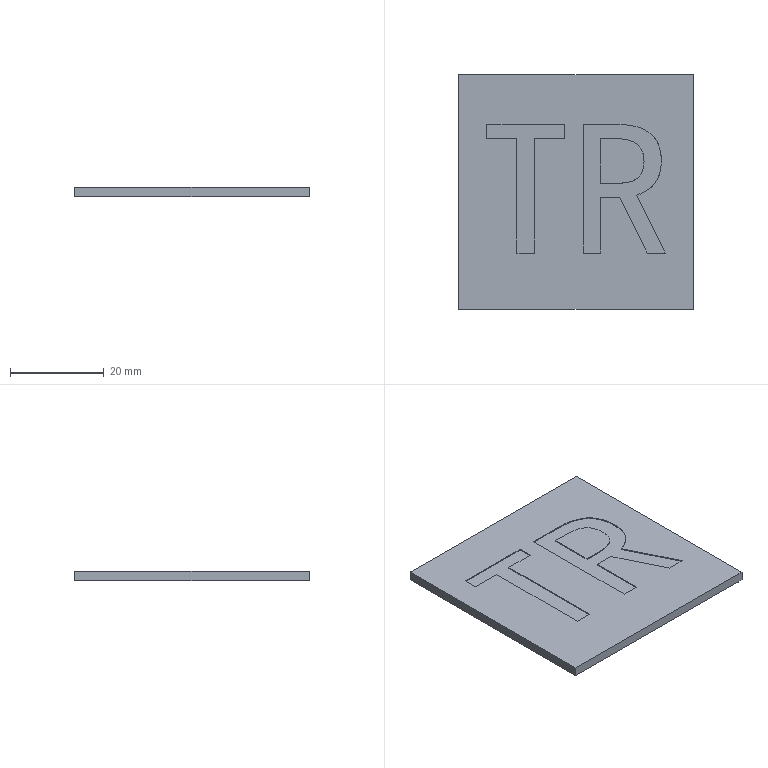Part | STEP file | lll_id986_x_t | 1 solid | 28 faces | box 50 x 50 x 2 mm | volume 4923 mm3 | plane 25 | other 3
STEP:
#1=CARTESIAN_POINT('',(645.037,-531.694,3.259));
#2=VERTEX_POINT('',#1);
#3=CARTESIAN_POINT('',(661.525,-531.694,3.259));
#4=VERTEX_POINT('',#3);
#5=CARTESIAN_POINT('',(653.281,-531.694,3.259));
#6=DIRECTION('',(1.,0.,0.));
#7=VECTOR('',#6,1.);
#8=LINE('',#5,#7);
#9=EDGE_CURVE('',#2,#4,#8,.T.);
#10=ORIENTED_EDGE('',*,*,#9,.T.);
#11=CARTESIAN_POINT('',(661.525,-534.734,3.259));
#12=VERTEX_POINT('',#11);
#13=CARTESIAN_POINT('',(661.525,-533.214,3.259));
#14=DIRECTION('',(0.,-1.,0.));
#15=VECTOR('',#14,1.);
#16=LINE('',#13,#15);
#17=EDGE_CURVE('',#4,#12,#16,.T.);
#18=ORIENTED_EDGE('',*,*,#17,.T.);
#19=CARTESIAN_POINT('',(655.124,-534.734,3.259));
#20=VERTEX_POINT('',#19);
#21=CARTESIAN_POINT('',(658.324,-534.734,3.259));
#22=DIRECTION('',(-1.,0.,0.));
#23=VECTOR('',#22,1.);
#24=LINE('',#21,#23);
#25=EDGE_CURVE('',#12,#20,#24,.T.);
#26=ORIENTED_EDGE('',*,*,#25,.T.);
#27=CARTESIAN_POINT('',(655.124,-559.065,3.259));
#28=VERTEX_POINT('',#27);
#29=CARTESIAN_POINT('',(655.124,-546.899,3.259));
#30=DIRECTION('',(0.,-1.,0.));
#31=VECTOR('',#30,1.);
#32=LINE('',#29,#31);
#33=EDGE_CURVE('',#20,#28,#32,.T.);
#34=ORIENTED_EDGE('',*,*,#33,.T.);
#35=CARTESIAN_POINT('',(651.439,-559.065,3.259));
#36=VERTEX_POINT('',#35);
#37=CARTESIAN_POINT('',(653.281,-559.065,3.259));
#38=DIRECTION('',(-1.,0.,0.));
#39=VECTOR('',#38,1.);
#40=LINE('',#37,#39);
#41=EDGE_CURVE('',#28,#36,#40,.T.);
#42=ORIENTED_EDGE('',*,*,#41,.T.);
#43=CARTESIAN_POINT('',(651.439,-534.734,3.259));
#44=VERTEX_POINT('',#43);
#45=CARTESIAN_POINT('',(651.439,-546.899,3.259));
#46=DIRECTION('',(0.,1.,0.));
#47=VECTOR('',#46,1.);
#48=LINE('',#45,#47);
#49=EDGE_CURVE('',#36,#44,#48,.T.);
#50=ORIENTED_EDGE('',*,*,#49,.T.);
#51=CARTESIAN_POINT('',(645.037,-534.734,3.259));
#52=VERTEX_POINT('',#51);
#53=CARTESIAN_POINT('',(648.238,-534.734,3.259));
#54=DIRECTION('',(-1.,0.,0.));
#55=VECTOR('',#54,1.);
#56=LINE('',#53,#55);
#57=EDGE_CURVE('',#44,#52,#56,.T.);
#58=ORIENTED_EDGE('',*,*,#57,.T.);
#59=CARTESIAN_POINT('',(645.037,-533.214,3.259));
#60=DIRECTION('',(0.,1.,0.));
#61=VECTOR('',#60,1.);
#62=LINE('',#59,#61);
#63=EDGE_CURVE('',#52,#2,#62,.T.);
#64=ORIENTED_EDGE('',*,*,#63,.T.);
#65=EDGE_LOOP('',(#10,#18,#26,#34,#42,#50,#58,#64));
#66=FACE_BOUND('',#65,.T.);
#67=CARTESIAN_POINT('',(689.009,-571.065,3.259));
#68=VERTEX_POINT('',#67);
#69=CARTESIAN_POINT('',(639.009,-571.065,3.259));
#70=VERTEX_POINT('',#69);
#71=CARTESIAN_POINT('',(739.009,-571.065,3.259));
#72=DIRECTION('',(-1.,0.,0.));
#73=VECTOR('',#72,1.);
#74=LINE('',#71,#73);
#75=EDGE_CURVE('',#68,#70,#74,.T.);
#76=ORIENTED_EDGE('',*,*,#75,.F.);
#77=CARTESIAN_POINT('',(689.009,-521.065,3.259));
#78=VERTEX_POINT('',#77);
#79=CARTESIAN_POINT('',(689.009,-471.065,3.259));
#80=DIRECTION('',(0.,-1.,0.));
#81=VECTOR('',#80,1.);
#82=LINE('',#79,#81);
#83=EDGE_CURVE('',#78,#68,#82,.T.);
#84=ORIENTED_EDGE('',*,*,#83,.F.);
#85=CARTESIAN_POINT('',(639.009,-521.065,3.259));
#86=VERTEX_POINT('',#85);
#87=CARTESIAN_POINT('',(739.009,-521.065,3.259));
#88=DIRECTION('',(-1.,0.,0.));
#89=VECTOR('',#88,1.);
#90=LINE('',#87,#89);
#91=EDGE_CURVE('',#78,#86,#90,.T.);
#92=ORIENTED_EDGE('',*,*,#91,.T.);
#93=CARTESIAN_POINT('',(639.009,-471.065,3.259));
#94=DIRECTION('',(0.,1.,0.));
#95=VECTOR('',#94,1.);
#96=LINE('',#93,#95);
#97=EDGE_CURVE('',#70,#86,#96,.T.);
#98=ORIENTED_EDGE('',*,*,#97,.F.);
#99=EDGE_LOOP('',(#76,#84,#92,#98));
#100=FACE_BOUND('',#99,.T.);
#101=CARTESIAN_POINT('',(665.533,-531.694,3.259));
#102=VERTEX_POINT('',#101);
#103=CARTESIAN_POINT('',(676.896,-546.742,3.259));
#104=VERTEX_POINT('',#103);
#105=CARTESIAN_POINT('',(665.533,-531.694,3.259));
#106=CARTESIAN_POINT('',(668.2,-531.694,3.259));
#107=CARTESIAN_POINT('',(670.867,-531.694,3.259));
#108=CARTESIAN_POINT('',(676.1,-531.694,3.259));
#109=CARTESIAN_POINT('',(678.179,-532.302,3.259));
#110=CARTESIAN_POINT('',(681.381,-534.767,3.259));
#111=CARTESIAN_POINT('',(682.179,-536.76,3.259));
#112=CARTESIAN_POINT('',(682.179,-541.668,3.259));
#113=CARTESIAN_POINT('',(681.646,-543.327,3.259));
#114=CARTESIAN_POINT('',(679.511,-545.673,3.259));
#115=CARTESIAN_POINT('',(678.284,-546.419,3.259));
#116=CARTESIAN_POINT('',(676.896,-546.742,3.259));
#117=B_SPLINE_CURVE_WITH_KNOTS('',3,(#105,#106,#107,#108,#109,#110,#111,#112,#113,#114,#115,#116),.UNSPECIFIED.,.F.,.F.,(4,2,2,2,2,4),(0.,0.2266,0.4448,0.6636,0.8315,1.),.UNSPECIFIED.);
#118=EDGE_CURVE('',#102,#104,#117,.T.);
#119=ORIENTED_EDGE('',*,*,#118,.T.);
#120=CARTESIAN_POINT('',(682.982,-559.065,3.259));
#121=VERTEX_POINT('',#120);
#122=CARTESIAN_POINT('',(679.939,-552.903,3.259));
#123=DIRECTION('',(0.4428,-0.8966,0.));
#124=VECTOR('',#123,1.);
#125=LINE('',#122,#124);
#126=EDGE_CURVE('',#104,#121,#125,.T.);
#127=ORIENTED_EDGE('',*,*,#126,.T.);
#128=CARTESIAN_POINT('',(679.14,-559.065,3.259));
#129=VERTEX_POINT('',#128);
#130=CARTESIAN_POINT('',(681.061,-559.065,3.259));
#131=DIRECTION('',(-1.,0.,0.));
#132=VECTOR('',#131,1.);
#133=LINE('',#130,#132);
#134=EDGE_CURVE('',#121,#129,#133,.T.);
#135=ORIENTED_EDGE('',*,*,#134,.T.);
#136=CARTESIAN_POINT('',(673.376,-547.222,3.259));
#137=VERTEX_POINT('',#136);
#138=CARTESIAN_POINT('',(676.258,-553.143,3.259));
#139=DIRECTION('',(-0.4376,0.8992,0.));
#140=VECTOR('',#139,1.);
#141=LINE('',#138,#140);
#142=EDGE_CURVE('',#129,#137,#141,.T.);
#143=ORIENTED_EDGE('',*,*,#142,.T.);
#144=CARTESIAN_POINT('',(669.21,-547.222,3.259));
#145=VERTEX_POINT('',#144);
#146=CARTESIAN_POINT('',(671.293,-547.222,3.259));
#147=DIRECTION('',(-1.,0.,0.));
#148=VECTOR('',#147,1.);
#149=LINE('',#146,#148);
#150=EDGE_CURVE('',#137,#145,#149,.T.);
#151=ORIENTED_EDGE('',*,*,#150,.T.);
#152=CARTESIAN_POINT('',(669.21,-559.065,3.259));
#153=VERTEX_POINT('',#152);
#154=CARTESIAN_POINT('',(669.21,-553.143,3.259));
#155=DIRECTION('',(0.,-1.,0.));
#156=VECTOR('',#155,1.);
#157=LINE('',#154,#156);
#158=EDGE_CURVE('',#145,#153,#157,.T.);
#159=ORIENTED_EDGE('',*,*,#158,.T.);
#160=CARTESIAN_POINT('',(665.533,-559.065,3.259));
#161=VERTEX_POINT('',#160);
#162=CARTESIAN_POINT('',(667.372,-559.065,3.259));
#163=DIRECTION('',(-1.,0.,0.));
#164=VECTOR('',#163,1.);
#165=LINE('',#162,#164);
#166=EDGE_CURVE('',#153,#161,#165,.T.);
#167=ORIENTED_EDGE('',*,*,#166,.T.);
#168=CARTESIAN_POINT('',(665.533,-545.38,3.259));
#169=DIRECTION('',(0.,1.,0.));
#170=VECTOR('',#169,1.);
#171=LINE('',#168,#170);
#172=EDGE_CURVE('',#161,#102,#171,.T.);
#173=ORIENTED_EDGE('',*,*,#172,.T.);
#174=EDGE_LOOP('',(#119,#127,#135,#143,#151,#159,#167,#173));
#175=FACE_BOUND('',#174,.T.);
#176=CARTESIAN_POINT('',(739.009,-471.065,3.259));
#177=DIRECTION('',(0.,0.,1.));
#178=DIRECTION('',(1.,0.,0.));
#179=AXIS2_PLACEMENT_3D('',#176,#177,#178);
#180=PLANE('',#179);
#181=ADVANCED_FACE('',(#66,#100,#175),#180,.T.);
#182=CARTESIAN_POINT('',(689.009,-571.065,1.259));
#183=VERTEX_POINT('',#182);
#184=CARTESIAN_POINT('',(689.009,-571.065,179.534));
#185=DIRECTION('',(0.,0.,1.));
#186=VECTOR('',#185,1.);
#187=LINE('',#184,#186);
#188=EDGE_CURVE('',#183,#68,#187,.T.);
#189=ORIENTED_EDGE('',*,*,#188,.F.);
#190=CARTESIAN_POINT('',(689.009,-521.065,1.259));
#191=VERTEX_POINT('',#190);
#192=CARTESIAN_POINT('',(689.009,-471.065,1.259));
#193=DIRECTION('',(0.,-1.,0.));
#194=VECTOR('',#193,1.);
#195=LINE('',#192,#194);
#196=EDGE_CURVE('',#191,#183,#195,.T.);
#197=ORIENTED_EDGE('',*,*,#196,.F.);
#198=CARTESIAN_POINT('',(689.009,-521.065,2.109));
#199=DIRECTION('',(0.,0.,-1.));
#200=VECTOR('',#199,1.);
#201=LINE('',#198,#200);
#202=EDGE_CURVE('',#78,#191,#201,.T.);
#203=ORIENTED_EDGE('',*,*,#202,.F.);
#204=ORIENTED_EDGE('',*,*,#83,.T.);
#205=EDGE_LOOP('',(#189,#197,#203,#204));
#206=FACE_OUTER_BOUND('',#205,.T.);
#207=CARTESIAN_POINT('',(689.009,-546.065,2.259));
#208=DIRECTION('',(1.,0.,0.));
#209=DIRECTION('',(0.,0.,-1.));
#210=AXIS2_PLACEMENT_3D('',#207,#208,#209);
#211=PLANE('',#210);
#212=ADVANCED_FACE('',(#206),#211,.T.);
#213=CARTESIAN_POINT('',(639.009,-521.065,1.259));
#214=VERTEX_POINT('',#213);
#215=CARTESIAN_POINT('',(639.009,-521.065,2.109));
#216=DIRECTION('',(0.,0.,1.));
#217=VECTOR('',#216,1.);
#218=LINE('',#215,#217);
#219=EDGE_CURVE('',#214,#86,#218,.T.);
#220=ORIENTED_EDGE('',*,*,#219,.F.);
#221=CARTESIAN_POINT('',(639.009,-571.065,1.259));
#222=VERTEX_POINT('',#221);
#223=CARTESIAN_POINT('',(639.009,-471.065,1.259));
#224=DIRECTION('',(0.,-1.,0.));
#225=VECTOR('',#224,1.);
#226=LINE('',#223,#225);
#227=EDGE_CURVE('',#214,#222,#226,.T.);
#228=ORIENTED_EDGE('',*,*,#227,.T.);
#229=CARTESIAN_POINT('',(639.009,-571.065,179.534));
#230=DIRECTION('',(0.,0.,1.));
#231=VECTOR('',#230,1.);
#232=LINE('',#229,#231);
#233=EDGE_CURVE('',#222,#70,#232,.T.);
#234=ORIENTED_EDGE('',*,*,#233,.T.);
#235=ORIENTED_EDGE('',*,*,#97,.T.);
#236=EDGE_LOOP('',(#220,#228,#234,#235));
#237=FACE_OUTER_BOUND('',#236,.T.);
#238=CARTESIAN_POINT('',(639.009,-521.065,2.109));
#239=DIRECTION('',(1.,0.,0.));
#240=DIRECTION('',(0.,0.,-1.));
#241=AXIS2_PLACEMENT_3D('',#238,#239,#240);
#242=PLANE('',#241);
#243=ADVANCED_FACE('',(#237),#242,.F.);
#244=ORIENTED_EDGE('',*,*,#91,.F.);
#245=ORIENTED_EDGE('',*,*,#202,.T.);
#246=CARTESIAN_POINT('',(-820.991,-521.065,1.259));
#247=DIRECTION('',(1.,0.,0.));
#248=VECTOR('',#247,1.);
#249=LINE('',#246,#248);
#250=EDGE_CURVE('',#214,#191,#249,.T.);
#251=ORIENTED_EDGE('',*,*,#250,.F.);
#252=ORIENTED_EDGE('',*,*,#219,.T.);
#253=EDGE_LOOP('',(#244,#245,#251,#252));
#254=FACE_OUTER_BOUND('',#253,.T.);
#255=CARTESIAN_POINT('',(689.009,-521.065,2.109));
#256=DIRECTION('',(0.,1.,0.));
#257=DIRECTION('',(0.,0.,1.));
#258=AXIS2_PLACEMENT_3D('',#255,#256,#257);
#259=PLANE('',#258);
#260=ADVANCED_FACE('',(#254),#259,.T.);
#261=CARTESIAN_POINT('',(-6577.12,-571.065,1.259));
#262=DIRECTION('',(1.,0.,0.));
#263=VECTOR('',#262,1.);
#264=LINE('',#261,#263);
#265=EDGE_CURVE('',#222,#183,#264,.T.);
#266=ORIENTED_EDGE('',*,*,#265,.T.);
#267=ORIENTED_EDGE('',*,*,#188,.T.);
#268=ORIENTED_EDGE('',*,*,#75,.T.);
#269=ORIENTED_EDGE('',*,*,#233,.F.);
#270=EDGE_LOOP('',(#266,#267,#268,#269));
#271=FACE_OUTER_BOUND('',#270,.T.);
#272=CARTESIAN_POINT('',(-6577.12,-571.065,179.534));
#273=DIRECTION('',(0.,-1.,0.));
#274=DIRECTION('',(0.,0.,-1.));
#275=AXIS2_PLACEMENT_3D('',#272,#273,#274);
#276=PLANE('',#275);
#277=ADVANCED_FACE('',(#271),#276,.T.);
#278=ORIENTED_EDGE('',*,*,#250,.T.);
#279=ORIENTED_EDGE('',*,*,#196,.T.);
#280=ORIENTED_EDGE('',*,*,#265,.F.);
#281=ORIENTED_EDGE('',*,*,#227,.F.);
#282=EDGE_LOOP('',(#278,#279,#280,#281));
#283=FACE_OUTER_BOUND('',#282,.T.);
#284=CARTESIAN_POINT('',(-820.991,-471.065,1.259));
#285=DIRECTION('',(0.,0.,-1.));
#286=DIRECTION('',(-1.,0.,0.));
#287=AXIS2_PLACEMENT_3D('',#284,#285,#286);
#288=PLANE('',#287);
#289=ADVANCED_FACE('',(#283),#288,.T.);
#290=ORIENTED_EDGE('',*,*,#17,.F.);
#291=CARTESIAN_POINT('',(661.525,-531.694,3.059));
#292=VERTEX_POINT('',#291);
#293=CARTESIAN_POINT('',(661.525,-531.694,3.059));
#294=DIRECTION('',(0.,0.,-1.));
#295=VECTOR('',#294,1.);
#296=LINE('',#293,#295);
#297=EDGE_CURVE('',#4,#292,#296,.T.);
#298=ORIENTED_EDGE('',*,*,#297,.T.);
#299=CARTESIAN_POINT('',(661.525,-534.734,3.059));
#300=VERTEX_POINT('',#299);
#301=CARTESIAN_POINT('',(661.525,-533.214,3.059));
#302=DIRECTION('',(0.,1.,0.));
#303=VECTOR('',#302,1.);
#304=LINE('',#301,#303);
#305=EDGE_CURVE('',#300,#292,#304,.T.);
#306=ORIENTED_EDGE('',*,*,#305,.F.);
#307=CARTESIAN_POINT('',(661.525,-534.734,3.059));
#308=DIRECTION('',(0.,0.,-1.));
#309=VECTOR('',#308,1.);
#310=LINE('',#307,#309);
#311=EDGE_CURVE('',#12,#300,#310,.T.);
#312=ORIENTED_EDGE('',*,*,#311,.F.);
#313=EDGE_LOOP('',(#290,#298,#306,#312));
#314=FACE_OUTER_BOUND('',#313,.T.);
#315=CARTESIAN_POINT('',(661.525,-531.694,3.059));
#316=DIRECTION('',(-1.,0.,0.));
#317=DIRECTION('',(0.,0.,1.));
#318=AXIS2_PLACEMENT_3D('',#315,#316,#317);
#319=PLANE('',#318);
#320=ADVANCED_FACE('',(#314),#319,.T.);
#321=ORIENTED_EDGE('',*,*,#25,.F.);
#322=ORIENTED_EDGE('',*,*,#311,.T.);
#323=CARTESIAN_POINT('',(655.124,-534.734,3.059));
#324=VERTEX_POINT('',#323);
#325=CARTESIAN_POINT('',(658.324,-534.734,3.059));
#326=DIRECTION('',(1.,0.,0.));
#327=VECTOR('',#326,1.);
#328=LINE('',#325,#327);
#329=EDGE_CURVE('',#324,#300,#328,.T.);
#330=ORIENTED_EDGE('',*,*,#329,.F.);
#331=CARTESIAN_POINT('',(655.124,-534.734,3.059));
#332=DIRECTION('',(0.,0.,-1.));
#333=VECTOR('',#332,1.);
#334=LINE('',#331,#333);
#335=EDGE_CURVE('',#20,#324,#334,.T.);
#336=ORIENTED_EDGE('',*,*,#335,.F.);
#337=EDGE_LOOP('',(#321,#322,#330,#336));
#338=FACE_OUTER_BOUND('',#337,.T.);
#339=CARTESIAN_POINT('',(661.525,-534.734,3.059));
#340=DIRECTION('',(0.,1.,0.));
#341=DIRECTION('',(0.,0.,1.));
#342=AXIS2_PLACEMENT_3D('',#339,#340,#341);
#343=PLANE('',#342);
#344=ADVANCED_FACE('',(#338),#343,.T.);
#345=ORIENTED_EDGE('',*,*,#33,.F.);
#346=ORIENTED_EDGE('',*,*,#335,.T.);
#347=CARTESIAN_POINT('',(655.124,-559.065,3.059));
#348=VERTEX_POINT('',#347);
#349=CARTESIAN_POINT('',(655.124,-546.899,3.059));
#350=DIRECTION('',(0.,1.,0.));
#351=VECTOR('',#350,1.);
#352=LINE('',#349,#351);
#353=EDGE_CURVE('',#348,#324,#352,.T.);
#354=ORIENTED_EDGE('',*,*,#353,.F.);
#355=CARTESIAN_POINT('',(655.124,-559.065,3.059));
#356=DIRECTION('',(0.,0.,-1.));
#357=VECTOR('',#356,1.);
#358=LINE('',#355,#357);
#359=EDGE_CURVE('',#28,#348,#358,.T.);
#360=ORIENTED_EDGE('',*,*,#359,.F.);
#361=EDGE_LOOP('',(#345,#346,#354,#360));
#362=FACE_OUTER_BOUND('',#361,.T.);
#363=CARTESIAN_POINT('',(655.124,-534.734,3.059));
#364=DIRECTION('',(-1.,0.,0.));
#365=DIRECTION('',(0.,0.,1.));
#366=AXIS2_PLACEMENT_3D('',#363,#364,#365);
#367=PLANE('',#366);
#368=ADVANCED_FACE('',(#362),#367,.T.);
#369=ORIENTED_EDGE('',*,*,#41,.F.);
#370=ORIENTED_EDGE('',*,*,#359,.T.);
#371=CARTESIAN_POINT('',(651.439,-559.065,3.059));
#372=VERTEX_POINT('',#371);
#373=CARTESIAN_POINT('',(653.281,-559.065,3.059));
#374=DIRECTION('',(1.,0.,0.));
#375=VECTOR('',#374,1.);
#376=LINE('',#373,#375);
#377=EDGE_CURVE('',#372,#348,#376,.T.);
#378=ORIENTED_EDGE('',*,*,#377,.F.);
#379=CARTESIAN_POINT('',(651.439,-559.065,3.059));
#380=DIRECTION('',(0.,0.,-1.));
#381=VECTOR('',#380,1.);
#382=LINE('',#379,#381);
#383=EDGE_CURVE('',#36,#372,#382,.T.);
#384=ORIENTED_EDGE('',*,*,#383,.F.);
#385=EDGE_LOOP('',(#369,#370,#378,#384));
#386=FACE_OUTER_BOUND('',#385,.T.);
#387=CARTESIAN_POINT('',(655.124,-559.065,3.059));
#388=DIRECTION('',(0.,1.,0.));
#389=DIRECTION('',(0.,0.,1.));
#390=AXIS2_PLACEMENT_3D('',#387,#388,#389);
#391=PLANE('',#390);
#392=ADVANCED_FACE('',(#386),#391,.T.);
#393=ORIENTED_EDGE('',*,*,#49,.F.);
#394=ORIENTED_EDGE('',*,*,#383,.T.);
#395=CARTESIAN_POINT('',(651.439,-534.734,3.059));
#396=VERTEX_POINT('',#395);
#397=CARTESIAN_POINT('',(651.439,-546.899,3.059));
#398=DIRECTION('',(0.,-1.,0.));
#399=VECTOR('',#398,1.);
#400=LINE('',#397,#399);
#401=EDGE_CURVE('',#396,#372,#400,.T.);
#402=ORIENTED_EDGE('',*,*,#401,.F.);
#403=CARTESIAN_POINT('',(651.439,-534.734,3.059));
#404=DIRECTION('',(0.,0.,-1.));
#405=VECTOR('',#404,1.);
#406=LINE('',#403,#405);
#407=EDGE_CURVE('',#44,#396,#406,.T.);
#408=ORIENTED_EDGE('',*,*,#407,.F.);
#409=EDGE_LOOP('',(#393,#394,#402,#408));
#410=FACE_OUTER_BOUND('',#409,.T.);
#411=CARTESIAN_POINT('',(651.439,-559.065,3.059));
#412=DIRECTION('',(1.,0.,0.));
#413=DIRECTION('',(0.,0.,-1.));
#414=AXIS2_PLACEMENT_3D('',#411,#412,#413);
#415=PLANE('',#414);
#416=ADVANCED_FACE('',(#410),#415,.T.);
#417=ORIENTED_EDGE('',*,*,#57,.F.);
#418=ORIENTED_EDGE('',*,*,#407,.T.);
#419=CARTESIAN_POINT('',(645.037,-534.734,3.059));
#420=VERTEX_POINT('',#419);
#421=CARTESIAN_POINT('',(648.238,-534.734,3.059));
#422=DIRECTION('',(1.,0.,0.));
#423=VECTOR('',#422,1.);
#424=LINE('',#421,#423);
#425=EDGE_CURVE('',#420,#396,#424,.T.);
#426=ORIENTED_EDGE('',*,*,#425,.F.);
#427=CARTESIAN_POINT('',(645.037,-534.734,3.059));
#428=DIRECTION('',(0.,0.,-1.));
#429=VECTOR('',#428,1.);
#430=LINE('',#427,#429);
#431=EDGE_CURVE('',#52,#420,#430,.T.);
#432=ORIENTED_EDGE('',*,*,#431,.F.);
#433=EDGE_LOOP('',(#417,#418,#426,#432));
#434=FACE_OUTER_BOUND('',#433,.T.);
#435=CARTESIAN_POINT('',(651.439,-534.734,3.059));
#436=DIRECTION('',(0.,1.,0.));
#437=DIRECTION('',(0.,0.,1.));
#438=AXIS2_PLACEMENT_3D('',#435,#436,#437);
#439=PLANE('',#438);
#440=ADVANCED_FACE('',(#434),#439,.T.);
#441=ORIENTED_EDGE('',*,*,#63,.F.);
#442=ORIENTED_EDGE('',*,*,#431,.T.);
#443=CARTESIAN_POINT('',(645.037,-531.694,3.059));
#444=VERTEX_POINT('',#443);
#445=CARTESIAN_POINT('',(645.037,-533.214,3.059));
#446=DIRECTION('',(0.,-1.,0.));
#447=VECTOR('',#446,1.);
#448=LINE('',#445,#447);
#449=EDGE_CURVE('',#444,#420,#448,.T.);
#450=ORIENTED_EDGE('',*,*,#449,.F.);
#451=CARTESIAN_POINT('',(645.037,-531.694,3.059));
#452=DIRECTION('',(0.,0.,-1.));
#453=VECTOR('',#452,1.);
#454=LINE('',#451,#453);
#455=EDGE_CURVE('',#2,#444,#454,.T.);
#456=ORIENTED_EDGE('',*,*,#455,.F.);
#457=EDGE_LOOP('',(#441,#442,#450,#456));
#458=FACE_OUTER_BOUND('',#457,.T.);
#459=CARTESIAN_POINT('',(645.037,-534.734,3.059));
#460=DIRECTION('',(1.,0.,0.));
#461=DIRECTION('',(0.,0.,-1.));
#462=AXIS2_PLACEMENT_3D('',#459,#460,#461);
#463=PLANE('',#462);
#464=ADVANCED_FACE('',(#458),#463,.T.);
#465=ORIENTED_EDGE('',*,*,#9,.F.);
#466=ORIENTED_EDGE('',*,*,#455,.T.);
#467=CARTESIAN_POINT('',(653.281,-531.694,3.059));
#468=DIRECTION('',(-1.,0.,0.));
#469=VECTOR('',#468,1.);
#470=LINE('',#467,#469);
#471=EDGE_CURVE('',#292,#444,#470,.T.);
#472=ORIENTED_EDGE('',*,*,#471,.F.);
#473=ORIENTED_EDGE('',*,*,#297,.F.);
#474=EDGE_LOOP('',(#465,#466,#472,#473));
#475=FACE_OUTER_BOUND('',#474,.T.);
#476=CARTESIAN_POINT('',(645.037,-531.694,3.059));
#477=DIRECTION('',(0.,-1.,0.));
#478=DIRECTION('',(0.,0.,-1.));
#479=AXIS2_PLACEMENT_3D('',#476,#477,#478);
#480=PLANE('',#479);
#481=ADVANCED_FACE('',(#475),#480,.T.);
#482=ORIENTED_EDGE('',*,*,#305,.T.);
#483=ORIENTED_EDGE('',*,*,#471,.T.);
#484=ORIENTED_EDGE('',*,*,#449,.T.);
#485=ORIENTED_EDGE('',*,*,#425,.T.);
#486=ORIENTED_EDGE('',*,*,#401,.T.);
#487=ORIENTED_EDGE('',*,*,#377,.T.);
#488=ORIENTED_EDGE('',*,*,#353,.T.);
#489=ORIENTED_EDGE('',*,*,#329,.T.);
#490=EDGE_LOOP('',(#482,#483,#484,#485,#486,#487,#488,#489));
#491=FACE_OUTER_BOUND('',#490,.T.);
#492=CARTESIAN_POINT('',(661.525,-533.214,3.059));
#493=DIRECTION('',(0.,0.,1.));
#494=DIRECTION('',(1.,0.,0.));
#495=AXIS2_PLACEMENT_3D('',#492,#493,#494);
#496=PLANE('',#495);
#497=ADVANCED_FACE('',(#491),#496,.T.);
#498=CARTESIAN_POINT('',(677.061,-543.139,3.259));
#499=VERTEX_POINT('',#498);
#500=CARTESIAN_POINT('',(669.21,-534.734,3.259));
#501=VERTEX_POINT('',#500);
#502=CARTESIAN_POINT('',(677.061,-543.139,3.259));
#503=CARTESIAN_POINT('',(678.021,-542.449,3.259));
#504=CARTESIAN_POINT('',(678.502,-541.248,3.259));
#505=CARTESIAN_POINT('',(678.502,-538.043,3.259));
#506=CARTESIAN_POINT('',(678.044,-536.865,3.259));
#507=CARTESIAN_POINT('',(676.224,-535.165,3.259));
#508=CARTESIAN_POINT('',(674.764,-534.734,3.259));
#509=CARTESIAN_POINT('',(671.562,-534.734,3.259));
#510=CARTESIAN_POINT('',(670.386,-534.734,3.259));
#511=CARTESIAN_POINT('',(669.21,-534.734,3.259));
#512=B_SPLINE_CURVE_WITH_KNOTS('',3,(#502,#503,#504,#505,#506,#507,#508,#509,#510,#511),.UNSPECIFIED.,.F.,.F.,(4,2,2,2,4),(0.,0.307,0.5749,0.8439,1.),.UNSPECIFIED.);
#513=EDGE_CURVE('',#499,#501,#512,.T.);
#514=ORIENTED_EDGE('',*,*,#513,.F.);
#515=CARTESIAN_POINT('',(677.061,-543.139,3.059));
#516=VERTEX_POINT('',#515);
#517=CARTESIAN_POINT('',(677.061,-543.139,3.059));
#518=DIRECTION('',(0.,0.,-1.));
#519=VECTOR('',#518,1.);
#520=LINE('',#517,#519);
#521=EDGE_CURVE('',#499,#516,#520,.T.);
#522=ORIENTED_EDGE('',*,*,#521,.T.);
#523=CARTESIAN_POINT('',(669.21,-534.734,3.059));
#524=VERTEX_POINT('',#523);
#525=CARTESIAN_POINT('',(669.21,-534.734,3.059));
#526=CARTESIAN_POINT('',(670.386,-534.734,3.059));
#527=CARTESIAN_POINT('',(671.562,-534.734,3.059));
#528=CARTESIAN_POINT('',(674.764,-534.734,3.059));
#529=CARTESIAN_POINT('',(676.224,-535.165,3.059));
#530=CARTESIAN_POINT('',(678.044,-536.865,3.059));
#531=CARTESIAN_POINT('',(678.502,-538.043,3.059));
#532=CARTESIAN_POINT('',(678.502,-541.248,3.059));
#533=CARTESIAN_POINT('',(678.021,-542.449,3.059));
#534=CARTESIAN_POINT('',(677.061,-543.139,3.059));
#535=B_SPLINE_CURVE_WITH_KNOTS('',3,(#525,#526,#527,#528,#529,#530,#531,#532,#533,#534),.UNSPECIFIED.,.F.,.F.,(4,2,2,2,4),(0.,0.1561,0.4251,0.693,1.),.UNSPECIFIED.);
#536=EDGE_CURVE('',#524,#516,#535,.T.);
#537=ORIENTED_EDGE('',*,*,#536,.F.);
#538=CARTESIAN_POINT('',(669.21,-534.734,3.059));
#539=DIRECTION('',(0.,0.,-1.));
#540=VECTOR('',#539,1.);
#541=LINE('',#538,#540);
#542=EDGE_CURVE('',#501,#524,#541,.T.);
#543=ORIENTED_EDGE('',*,*,#542,.F.);
#544=EDGE_LOOP('',(#514,#522,#537,#543));
#545=FACE_OUTER_BOUND('',#544,.T.);
#546=CARTESIAN_POINT('',(677.061,-543.139,3.059));
#547=CARTESIAN_POINT('',(678.021,-542.449,3.059));
#548=CARTESIAN_POINT('',(678.502,-541.248,3.059));
#549=CARTESIAN_POINT('',(678.502,-538.043,3.059));
#550=CARTESIAN_POINT('',(678.044,-536.865,3.059));
#551=CARTESIAN_POINT('',(676.224,-535.165,3.059));
#552=CARTESIAN_POINT('',(674.764,-534.734,3.059));
#553=CARTESIAN_POINT('',(671.562,-534.734,3.059));
#554=CARTESIAN_POINT('',(670.386,-534.734,3.059));
#555=CARTESIAN_POINT('',(669.21,-534.734,3.059));
#556=B_SPLINE_CURVE_WITH_KNOTS('',3,(#546,#547,#548,#549,#550,#551,#552,#553,#554,#555),.UNSPECIFIED.,.F.,.F.,(4,2,2,2,4),(0.,0.307,0.5749,0.8439,1.),.UNSPECIFIED.);
#557=DIRECTION('',(0.,0.,1.));
#558=VECTOR('',#557,1.);
#559=SURFACE_OF_LINEAR_EXTRUSION('',#556,#558);
#560=ADVANCED_FACE('',(#545),#559,.T.);
#561=CARTESIAN_POINT('',(669.21,-544.182,3.259));
#562=VERTEX_POINT('',#561);
#563=CARTESIAN_POINT('',(669.21,-539.458,3.259));
#564=DIRECTION('',(0.,-1.,0.));
#565=VECTOR('',#564,1.);
#566=LINE('',#563,#565);
#567=EDGE_CURVE('',#501,#562,#566,.T.);
#568=ORIENTED_EDGE('',*,*,#567,.F.);
#569=ORIENTED_EDGE('',*,*,#542,.T.);
#570=CARTESIAN_POINT('',(669.21,-544.182,3.059));
#571=VERTEX_POINT('',#570);
#572=CARTESIAN_POINT('',(669.21,-539.458,3.059));
#573=DIRECTION('',(0.,1.,0.));
#574=VECTOR('',#573,1.);
#575=LINE('',#572,#574);
#576=EDGE_CURVE('',#571,#524,#575,.T.);
#577=ORIENTED_EDGE('',*,*,#576,.F.);
#578=CARTESIAN_POINT('',(669.21,-544.182,3.059));
#579=DIRECTION('',(0.,0.,-1.));
#580=VECTOR('',#579,1.);
#581=LINE('',#578,#580);
#582=EDGE_CURVE('',#562,#571,#581,.T.);
#583=ORIENTED_EDGE('',*,*,#582,.F.);
#584=EDGE_LOOP('',(#568,#569,#577,#583));
#585=FACE_OUTER_BOUND('',#584,.T.);
#586=CARTESIAN_POINT('',(669.21,-534.734,3.059));
#587=DIRECTION('',(-1.,0.,0.));
#588=DIRECTION('',(0.,0.,1.));
#589=AXIS2_PLACEMENT_3D('',#586,#587,#588);
#590=PLANE('',#589);
#591=ADVANCED_FACE('',(#585),#590,.T.);
#592=ORIENTED_EDGE('',*,*,#126,.F.);
#593=CARTESIAN_POINT('',(676.896,-546.742,3.059));
#594=VERTEX_POINT('',#593);
#595=CARTESIAN_POINT('',(676.896,-546.742,3.059));
#596=DIRECTION('',(0.,0.,-1.));
#597=VECTOR('',#596,1.);
#598=LINE('',#595,#597);
#599=EDGE_CURVE('',#104,#594,#598,.T.);
#600=ORIENTED_EDGE('',*,*,#599,.T.);
#601=CARTESIAN_POINT('',(682.982,-559.065,3.059));
#602=VERTEX_POINT('',#601);
#603=CARTESIAN_POINT('',(679.939,-552.903,3.059));
#604=DIRECTION('',(-0.4428,0.8966,0.));
#605=VECTOR('',#604,1.);
#606=LINE('',#603,#605);
#607=EDGE_CURVE('',#602,#594,#606,.T.);
#608=ORIENTED_EDGE('',*,*,#607,.F.);
#609=CARTESIAN_POINT('',(682.982,-559.065,3.059));
#610=DIRECTION('',(0.,0.,-1.));
#611=VECTOR('',#610,1.);
#612=LINE('',#609,#611);
#613=EDGE_CURVE('',#121,#602,#612,.T.);
#614=ORIENTED_EDGE('',*,*,#613,.F.);
#615=EDGE_LOOP('',(#592,#600,#608,#614));
#616=FACE_OUTER_BOUND('',#615,.T.);
#617=CARTESIAN_POINT('',(676.896,-546.742,3.059));
#618=DIRECTION('',(-0.8966,-0.4428,0.));
#619=DIRECTION('',(0.4428,-0.8966,0.));
#620=AXIS2_PLACEMENT_3D('',#617,#618,#619);
#621=PLANE('',#620);
#622=ADVANCED_FACE('',(#616),#621,.T.);
#623=ORIENTED_EDGE('',*,*,#134,.F.);
#624=ORIENTED_EDGE('',*,*,#613,.T.);
#625=CARTESIAN_POINT('',(679.14,-559.065,3.059));
#626=VERTEX_POINT('',#625);
#627=CARTESIAN_POINT('',(681.061,-559.065,3.059));
#628=DIRECTION('',(1.,0.,0.));
#629=VECTOR('',#628,1.);
#630=LINE('',#627,#629);
#631=EDGE_CURVE('',#626,#602,#630,.T.);
#632=ORIENTED_EDGE('',*,*,#631,.F.);
#633=CARTESIAN_POINT('',(679.14,-559.065,3.059));
#634=DIRECTION('',(0.,0.,-1.));
#635=VECTOR('',#634,1.);
#636=LINE('',#633,#635);
#637=EDGE_CURVE('',#129,#626,#636,.T.);
#638=ORIENTED_EDGE('',*,*,#637,.F.);
#639=EDGE_LOOP('',(#623,#624,#632,#638));
#640=FACE_OUTER_BOUND('',#639,.T.);
#641=CARTESIAN_POINT('',(682.982,-559.065,3.059));
#642=DIRECTION('',(0.,1.,0.));
#643=DIRECTION('',(0.,0.,1.));
#644=AXIS2_PLACEMENT_3D('',#641,#642,#643);
#645=PLANE('',#644);
#646=ADVANCED_FACE('',(#640),#645,.T.);
#647=ORIENTED_EDGE('',*,*,#142,.F.);
#648=ORIENTED_EDGE('',*,*,#637,.T.);
#649=CARTESIAN_POINT('',(673.376,-547.222,3.059));
#650=VERTEX_POINT('',#649);
#651=CARTESIAN_POINT('',(676.258,-553.143,3.059));
#652=DIRECTION('',(0.4376,-0.8992,0.));
#653=VECTOR('',#652,1.);
#654=LINE('',#651,#653);
#655=EDGE_CURVE('',#650,#626,#654,.T.);
#656=ORIENTED_EDGE('',*,*,#655,.F.);
#657=CARTESIAN_POINT('',(673.376,-547.222,3.059));
#658=DIRECTION('',(0.,0.,-1.));
#659=VECTOR('',#658,1.);
#660=LINE('',#657,#659);
#661=EDGE_CURVE('',#137,#650,#660,.T.);
#662=ORIENTED_EDGE('',*,*,#661,.F.);
#663=EDGE_LOOP('',(#647,#648,#656,#662));
#664=FACE_OUTER_BOUND('',#663,.T.);
#665=CARTESIAN_POINT('',(679.14,-559.065,3.059));
#666=DIRECTION('',(0.8992,0.4376,0.));
#667=DIRECTION('',(-0.4376,0.8992,0.));
#668=AXIS2_PLACEMENT_3D('',#665,#666,#667);
#669=PLANE('',#668);
#670=ADVANCED_FACE('',(#664),#669,.T.);
#671=ORIENTED_EDGE('',*,*,#150,.F.);
#672=ORIENTED_EDGE('',*,*,#661,.T.);
#673=CARTESIAN_POINT('',(669.21,-547.222,3.059));
#674=VERTEX_POINT('',#673);
#675=CARTESIAN_POINT('',(671.293,-547.222,3.059));
#676=DIRECTION('',(1.,0.,0.));
#677=VECTOR('',#676,1.);
#678=LINE('',#675,#677);
#679=EDGE_CURVE('',#674,#650,#678,.T.);
#680=ORIENTED_EDGE('',*,*,#679,.F.);
#681=CARTESIAN_POINT('',(669.21,-547.222,3.059));
#682=DIRECTION('',(0.,0.,-1.));
#683=VECTOR('',#682,1.);
#684=LINE('',#681,#683);
#685=EDGE_CURVE('',#145,#674,#684,.T.);
#686=ORIENTED_EDGE('',*,*,#685,.F.);
#687=EDGE_LOOP('',(#671,#672,#680,#686));
#688=FACE_OUTER_BOUND('',#687,.T.);
#689=CARTESIAN_POINT('',(673.376,-547.222,3.059));
#690=DIRECTION('',(0.,1.,0.));
#691=DIRECTION('',(0.,0.,1.));
#692=AXIS2_PLACEMENT_3D('',#689,#690,#691);
#693=PLANE('',#692);
#694=ADVANCED_FACE('',(#688),#693,.T.);
#695=ORIENTED_EDGE('',*,*,#158,.F.);
#696=ORIENTED_EDGE('',*,*,#685,.T.);
#697=CARTESIAN_POINT('',(669.21,-559.065,3.059));
#698=VERTEX_POINT('',#697);
#699=CARTESIAN_POINT('',(669.21,-553.143,3.059));
#700=DIRECTION('',(0.,1.,0.));
#701=VECTOR('',#700,1.);
#702=LINE('',#699,#701);
#703=EDGE_CURVE('',#698,#674,#702,.T.);
#704=ORIENTED_EDGE('',*,*,#703,.F.);
#705=CARTESIAN_POINT('',(669.21,-559.065,3.059));
#706=DIRECTION('',(0.,0.,-1.));
#707=VECTOR('',#706,1.);
#708=LINE('',#705,#707);
#709=EDGE_CURVE('',#153,#698,#708,.T.);
#710=ORIENTED_EDGE('',*,*,#709,.F.);
#711=EDGE_LOOP('',(#695,#696,#704,#710));
#712=FACE_OUTER_BOUND('',#711,.T.);
#713=CARTESIAN_POINT('',(669.21,-547.222,3.059));
#714=DIRECTION('',(-1.,0.,0.));
#715=DIRECTION('',(0.,0.,1.));
#716=AXIS2_PLACEMENT_3D('',#713,#714,#715);
#717=PLANE('',#716);
#718=ADVANCED_FACE('',(#712),#717,.T.);
#719=ORIENTED_EDGE('',*,*,#166,.F.);
#720=ORIENTED_EDGE('',*,*,#709,.T.);
#721=CARTESIAN_POINT('',(665.533,-559.065,3.059));
#722=VERTEX_POINT('',#721);
#723=CARTESIAN_POINT('',(667.372,-559.065,3.059));
#724=DIRECTION('',(1.,0.,0.));
#725=VECTOR('',#724,1.);
#726=LINE('',#723,#725);
#727=EDGE_CURVE('',#722,#698,#726,.T.);
#728=ORIENTED_EDGE('',*,*,#727,.F.);
#729=CARTESIAN_POINT('',(665.533,-559.065,3.059));
#730=DIRECTION('',(0.,0.,-1.));
#731=VECTOR('',#730,1.);
#732=LINE('',#729,#731);
#733=EDGE_CURVE('',#161,#722,#732,.T.);
#734=ORIENTED_EDGE('',*,*,#733,.F.);
#735=EDGE_LOOP('',(#719,#720,#728,#734));
#736=FACE_OUTER_BOUND('',#735,.T.);
#737=CARTESIAN_POINT('',(669.21,-559.065,3.059));
#738=DIRECTION('',(0.,1.,0.));
#739=DIRECTION('',(0.,0.,1.));
#740=AXIS2_PLACEMENT_3D('',#737,#738,#739);
#741=PLANE('',#740);
#742=ADVANCED_FACE('',(#736),#741,.T.);
#743=ORIENTED_EDGE('',*,*,#172,.F.);
#744=ORIENTED_EDGE('',*,*,#733,.T.);
#745=CARTESIAN_POINT('',(665.533,-531.694,3.059));
#746=VERTEX_POINT('',#745);
#747=CARTESIAN_POINT('',(665.533,-545.38,3.059));
#748=DIRECTION('',(0.,-1.,0.));
#749=VECTOR('',#748,1.);
#750=LINE('',#747,#749);
#751=EDGE_CURVE('',#746,#722,#750,.T.);
#752=ORIENTED_EDGE('',*,*,#751,.F.);
#753=CARTESIAN_POINT('',(665.533,-531.694,3.059));
#754=DIRECTION('',(0.,0.,-1.));
#755=VECTOR('',#754,1.);
#756=LINE('',#753,#755);
#757=EDGE_CURVE('',#102,#746,#756,.T.);
#758=ORIENTED_EDGE('',*,*,#757,.F.);
#759=EDGE_LOOP('',(#743,#744,#752,#758));
#760=FACE_OUTER_BOUND('',#759,.T.);
#761=CARTESIAN_POINT('',(665.533,-559.065,3.059));
#762=DIRECTION('',(1.,0.,0.));
#763=DIRECTION('',(0.,0.,-1.));
#764=AXIS2_PLACEMENT_3D('',#761,#762,#763);
#765=PLANE('',#764);
#766=ADVANCED_FACE('',(#760),#765,.T.);
#767=ORIENTED_EDGE('',*,*,#118,.F.);
#768=ORIENTED_EDGE('',*,*,#757,.T.);
#769=CARTESIAN_POINT('',(676.896,-546.742,3.059));
#770=CARTESIAN_POINT('',(678.284,-546.419,3.059));
#771=CARTESIAN_POINT('',(679.511,-545.673,3.059));
#772=CARTESIAN_POINT('',(681.646,-543.327,3.059));
#773=CARTESIAN_POINT('',(682.179,-541.668,3.059));
#774=CARTESIAN_POINT('',(682.179,-536.76,3.059));
#775=CARTESIAN_POINT('',(681.381,-534.767,3.059));
#776=CARTESIAN_POINT('',(678.179,-532.302,3.059));
#777=CARTESIAN_POINT('',(676.1,-531.694,3.059));
#778=CARTESIAN_POINT('',(670.867,-531.694,3.059));
#779=CARTESIAN_POINT('',(668.2,-531.694,3.059));
#780=CARTESIAN_POINT('',(665.533,-531.694,3.059));
#781=B_SPLINE_CURVE_WITH_KNOTS('',3,(#769,#770,#771,#772,#773,#774,#775,#776,#777,#778,#779,#780),.UNSPECIFIED.,.F.,.F.,(4,2,2,2,2,4),(0.,0.1685,0.3364,0.5552,0.7734,1.),.UNSPECIFIED.);
#782=EDGE_CURVE('',#594,#746,#781,.T.);
#783=ORIENTED_EDGE('',*,*,#782,.F.);
#784=ORIENTED_EDGE('',*,*,#599,.F.);
#785=EDGE_LOOP('',(#767,#768,#783,#784));
#786=FACE_OUTER_BOUND('',#785,.T.);
#787=CARTESIAN_POINT('',(665.533,-531.694,3.059));
#788=CARTESIAN_POINT('',(668.2,-531.694,3.059));
#789=CARTESIAN_POINT('',(670.867,-531.694,3.059));
#790=CARTESIAN_POINT('',(676.1,-531.694,3.059));
#791=CARTESIAN_POINT('',(678.179,-532.302,3.059));
#792=CARTESIAN_POINT('',(681.381,-534.767,3.059));
#793=CARTESIAN_POINT('',(682.179,-536.76,3.059));
#794=CARTESIAN_POINT('',(682.179,-541.668,3.059));
#795=CARTESIAN_POINT('',(681.646,-543.327,3.059));
#796=CARTESIAN_POINT('',(679.511,-545.673,3.059));
#797=CARTESIAN_POINT('',(678.284,-546.419,3.059));
#798=CARTESIAN_POINT('',(676.896,-546.742,3.059));
#799=B_SPLINE_CURVE_WITH_KNOTS('',3,(#787,#788,#789,#790,#791,#792,#793,#794,#795,#796,#797,#798),.UNSPECIFIED.,.F.,.F.,(4,2,2,2,2,4),(0.,0.2266,0.4448,0.6636,0.8315,1.),.UNSPECIFIED.);
#800=DIRECTION('',(0.,0.,1.));
#801=VECTOR('',#800,1.);
#802=SURFACE_OF_LINEAR_EXTRUSION('',#799,#801);
#803=ADVANCED_FACE('',(#786),#802,.T.);
#804=CARTESIAN_POINT('',(669.21,-544.182,3.259));
#805=CARTESIAN_POINT('',(670.706,-544.182,3.259));
#806=CARTESIAN_POINT('',(672.202,-544.182,3.259));
#807=CARTESIAN_POINT('',(674.974,-544.182,3.259));
#808=CARTESIAN_POINT('',(676.1,-543.83,3.259));
#809=CARTESIAN_POINT('',(677.061,-543.139,3.259));
#810=B_SPLINE_CURVE_WITH_KNOTS('',3,(#804,#805,#806,#807,#808,#809),.UNSPECIFIED.,.F.,.F.,(4,2,4),(0.,0.5397,1.),.UNSPECIFIED.);
#811=EDGE_CURVE('',#562,#499,#810,.T.);
#812=ORIENTED_EDGE('',*,*,#811,.F.);
#813=ORIENTED_EDGE('',*,*,#582,.T.);
#814=CARTESIAN_POINT('',(677.061,-543.139,3.059));
#815=CARTESIAN_POINT('',(676.1,-543.83,3.059));
#816=CARTESIAN_POINT('',(674.974,-544.182,3.059));
#817=CARTESIAN_POINT('',(672.202,-544.182,3.059));
#818=CARTESIAN_POINT('',(670.706,-544.182,3.059));
#819=CARTESIAN_POINT('',(669.21,-544.182,3.059));
#820=B_SPLINE_CURVE_WITH_KNOTS('',3,(#814,#815,#816,#817,#818,#819),.UNSPECIFIED.,.F.,.F.,(4,2,4),(0.,0.4603,1.),.UNSPECIFIED.);
#821=EDGE_CURVE('',#516,#571,#820,.T.);
#822=ORIENTED_EDGE('',*,*,#821,.F.);
#823=ORIENTED_EDGE('',*,*,#521,.F.);
#824=EDGE_LOOP('',(#812,#813,#822,#823));
#825=FACE_OUTER_BOUND('',#824,.T.);
#826=CARTESIAN_POINT('',(669.21,-544.182,3.059));
#827=CARTESIAN_POINT('',(670.706,-544.182,3.059));
#828=CARTESIAN_POINT('',(672.202,-544.182,3.059));
#829=CARTESIAN_POINT('',(674.974,-544.182,3.059));
#830=CARTESIAN_POINT('',(676.1,-543.83,3.059));
#831=CARTESIAN_POINT('',(677.061,-543.139,3.059));
#832=B_SPLINE_CURVE_WITH_KNOTS('',3,(#826,#827,#828,#829,#830,#831),.UNSPECIFIED.,.F.,.F.,(4,2,4),(0.,0.5397,1.),.UNSPECIFIED.);
#833=DIRECTION('',(0.,0.,1.));
#834=VECTOR('',#833,1.);
#835=SURFACE_OF_LINEAR_EXTRUSION('',#832,#834);
#836=ADVANCED_FACE('',(#825),#835,.T.);
#837=ORIENTED_EDGE('',*,*,#607,.T.);
#838=ORIENTED_EDGE('',*,*,#782,.T.);
#839=ORIENTED_EDGE('',*,*,#751,.T.);
#840=ORIENTED_EDGE('',*,*,#727,.T.);
#841=ORIENTED_EDGE('',*,*,#703,.T.);
#842=ORIENTED_EDGE('',*,*,#679,.T.);
#843=ORIENTED_EDGE('',*,*,#655,.T.);
#844=ORIENTED_EDGE('',*,*,#631,.T.);
#845=EDGE_LOOP('',(#837,#838,#839,#840,#841,#842,#843,#844));
#846=FACE_BOUND('',#845,.T.);
#847=ORIENTED_EDGE('',*,*,#536,.T.);
#848=ORIENTED_EDGE('',*,*,#821,.T.);
#849=ORIENTED_EDGE('',*,*,#576,.T.);
#850=EDGE_LOOP('',(#847,#848,#849));
#851=FACE_BOUND('',#850,.T.);
#852=CARTESIAN_POINT('',(680.838,-534.613,3.059));
#853=DIRECTION('',(0.,0.,1.));
#854=DIRECTION('',(0.,-1.,0.));
#855=AXIS2_PLACEMENT_3D('',#852,#853,#854);
#856=PLANE('',#855);
#857=ADVANCED_FACE('',(#846,#851),#856,.T.);
#858=ORIENTED_EDGE('',*,*,#811,.T.);
#859=ORIENTED_EDGE('',*,*,#513,.T.);
#860=ORIENTED_EDGE('',*,*,#567,.T.);
#861=EDGE_LOOP('',(#858,#859,#860));
#862=FACE_OUTER_BOUND('',#861,.T.);
#863=CARTESIAN_POINT('',(739.009,-471.065,3.259));
#864=DIRECTION('',(0.,0.,1.));
#865=DIRECTION('',(1.,0.,0.));
#866=AXIS2_PLACEMENT_3D('',#863,#864,#865);
#867=PLANE('',#866);
#868=ADVANCED_FACE('',(#862),#867,.T.);
#869=CLOSED_SHELL('',(#181,#212,#243,#260,#277,#289,#320,#344,#368,#392,#416,#440,#464,#481,#497,#560,#591,#622,#646,#670,#694,#718,#742,#766,#803,#836,#857,#868));
#870=MANIFOLD_SOLID_BREP('',#869);
#871=(LENGTH_UNIT()NAMED_UNIT(*)SI_UNIT(.MILLI.,.METRE.));
#872=UNCERTAINTY_MEASURE_WITH_UNIT(LENGTH_MEASURE(0.00002),#871,'','');
#873=(NAMED_UNIT(*)PLANE_ANGLE_UNIT()SI_UNIT($,.RADIAN.));
#874=PLANE_ANGLE_MEASURE_WITH_UNIT(PLANE_ANGLE_MEASURE(0.01745),#873);
#875=DIMENSIONAL_EXPONENTS(0.,0.,0.,0.,0.,0.,0.);
#876=(CONVERSION_BASED_UNIT('DEGREE',#874)NAMED_UNIT(#875)PLANE_ANGLE_UNIT());
#877=(NAMED_UNIT(*)SI_UNIT($,.STERADIAN.)SOLID_ANGLE_UNIT());
#878=(GEOMETRIC_REPRESENTATION_CONTEXT(3)GLOBAL_UNCERTAINTY_ASSIGNED_CONTEXT((#872))GLOBAL_UNIT_ASSIGNED_CONTEXT((#871,#876,#877))REPRESENTATION_CONTEXT('',''));
#879=ADVANCED_BREP_SHAPE_REPRESENTATION('',(#870),#878);